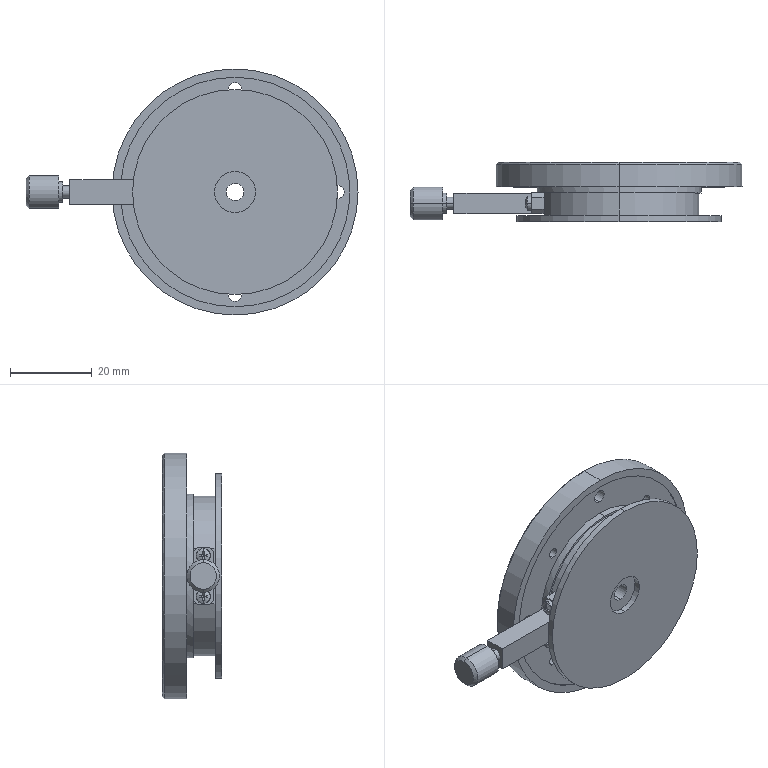Part | SolidWorks | features BaseBody 1 | 1 solid | 189 faces | box 81 x 14.5 x 60 mm | volume 28270 mm3 | plane 79 | cylinder 70 | cone 28 | spline 12 | commonest cylinder face diameters 2.5 x8 3.3 x8 3.5 x8 2 x7 32 x5 2.1 x4